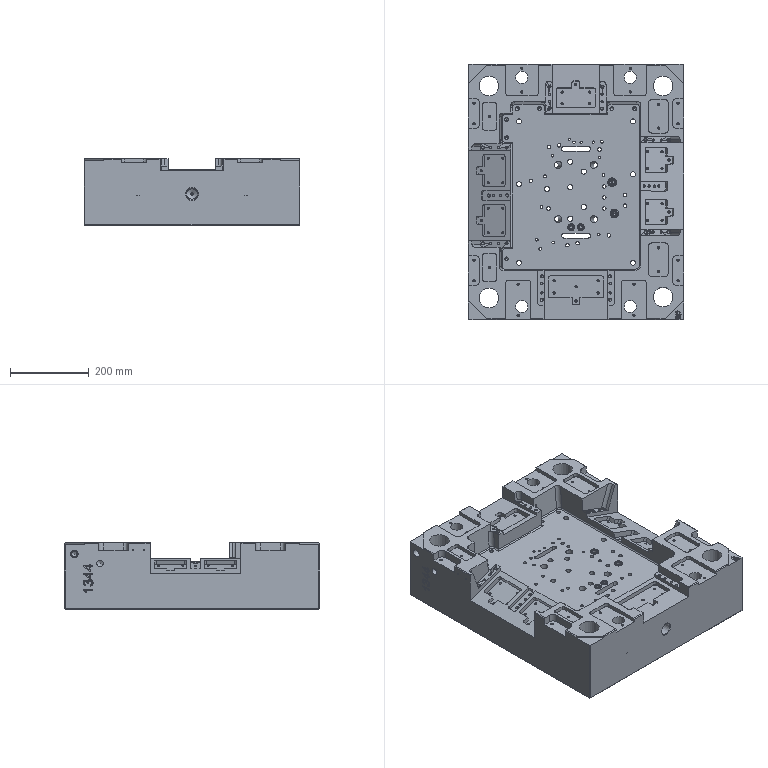Part | STEP file | P011002B001-000 | 1 solid | 3039 faces | volume 41496641 mm3 | plane 1526 | cylinder 574 | cone 523 | other 369 | spline 34 | torus 13 | commonest cylinder face diameters 6 x108 10 x71 5.98 x70 5 x69 8 x29 16 x28